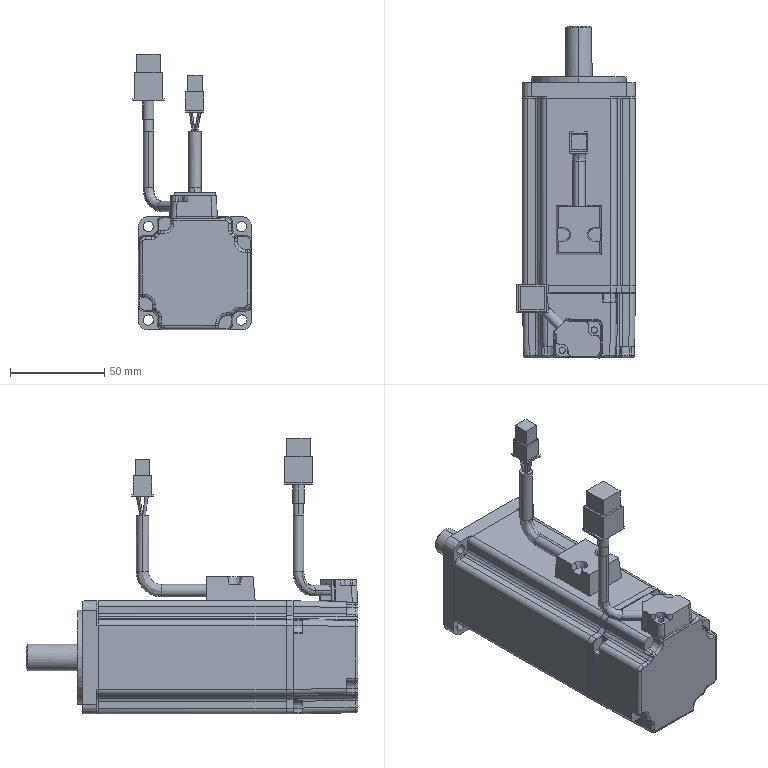Part | SolidWorks | features BaseBody 2 | 2 solids | 510 faces | box 63.089 x 175.904 x 146.235 mm | volume 489456 mm3 | plane 221 | cylinder 189 | cone 51 | spline 49 | commonest cylinder face diameters 6 x40 4 x32 3 x31 0.6 x12 1.5 x11 1 x10